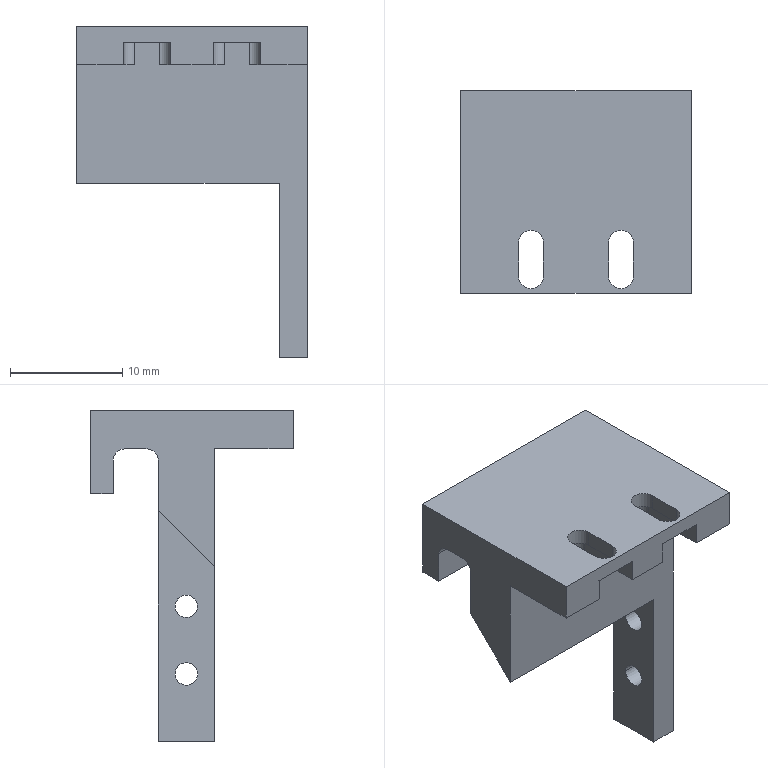NC program | NX | posted with a generic post | part box 20.5 x 18 x 29.4 mm
Lines 1 to 26 of 6588:
N10 G17 G21 G94 G90
(FLOOR_WALL , TOOL : D10JING)
N12 T09 M6
N14 G54
N16 G17 G0 G90 X-20.25 Y10.997 S9500 M3
N18 G43 Z30. H9
N20 Z3.
N22 G94 G1 Z0. F1250.
N24 X-17.25
N26 X17.25
N28 Y6.498
N30 X-17.25
N32 Y1.999
N34 X17.25
N36 Y-2.501
N38 X-17.25
N40 Y-7.
N42 X17.25
N44 X20.25
N46 Z3.
N48 G0 Z30.
N50 M5